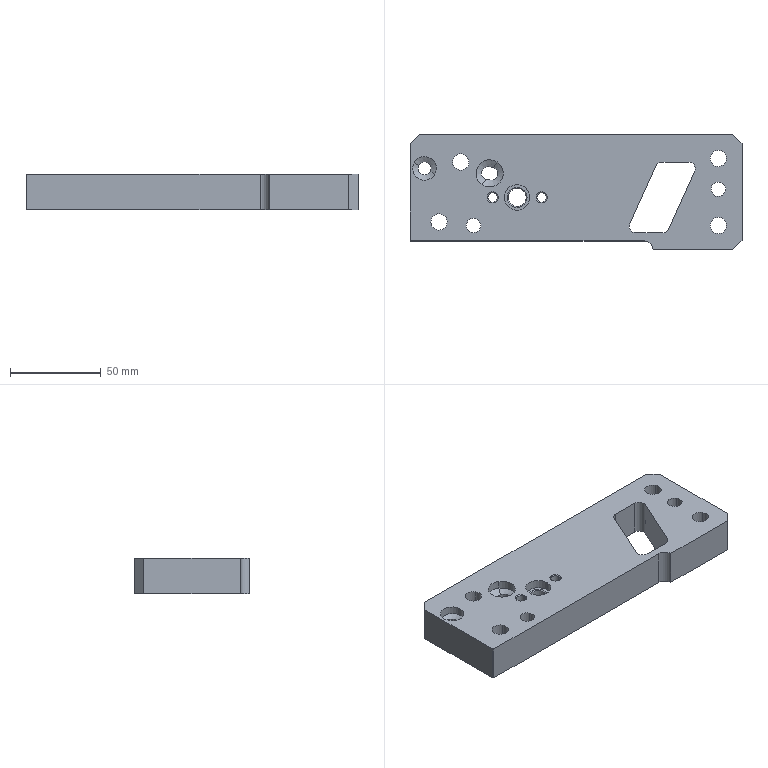Part | CATIA | 1 solid | 73 faces | box 183 x 63 x 19.5 mm | volume 178829 mm3 | cylinder 41 | plane 22 | cone 10 | commonest cylinder face diameters 15 x10 9 x8 5.2 x4 7 x4 7.2 x4 8 x4